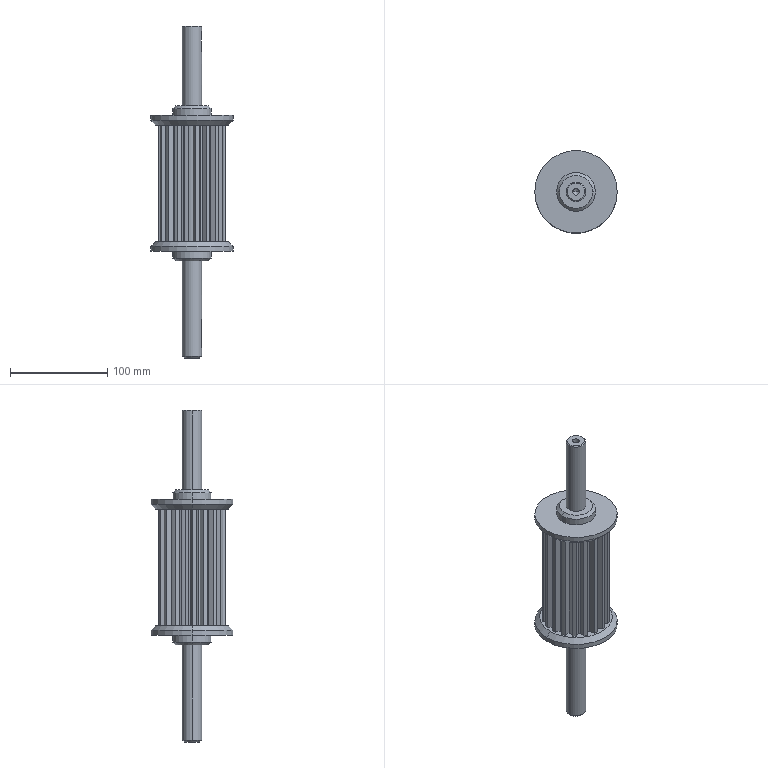Part | STEP file | Driving roller | 1 solid | 130 faces | box 85 x 85 x 342 mm | volume 592269 mm3 | cylinder 62 | plane 52 | cone 16 | commonest cylinder face diameters 60 x19 70 x19 6 x8 6.8 x4 20 x4 40 x4